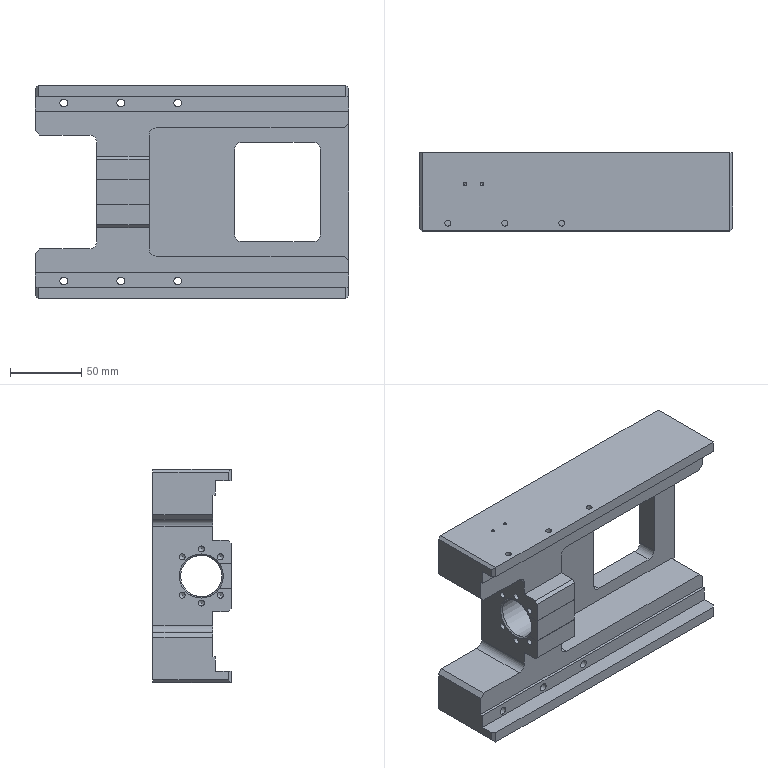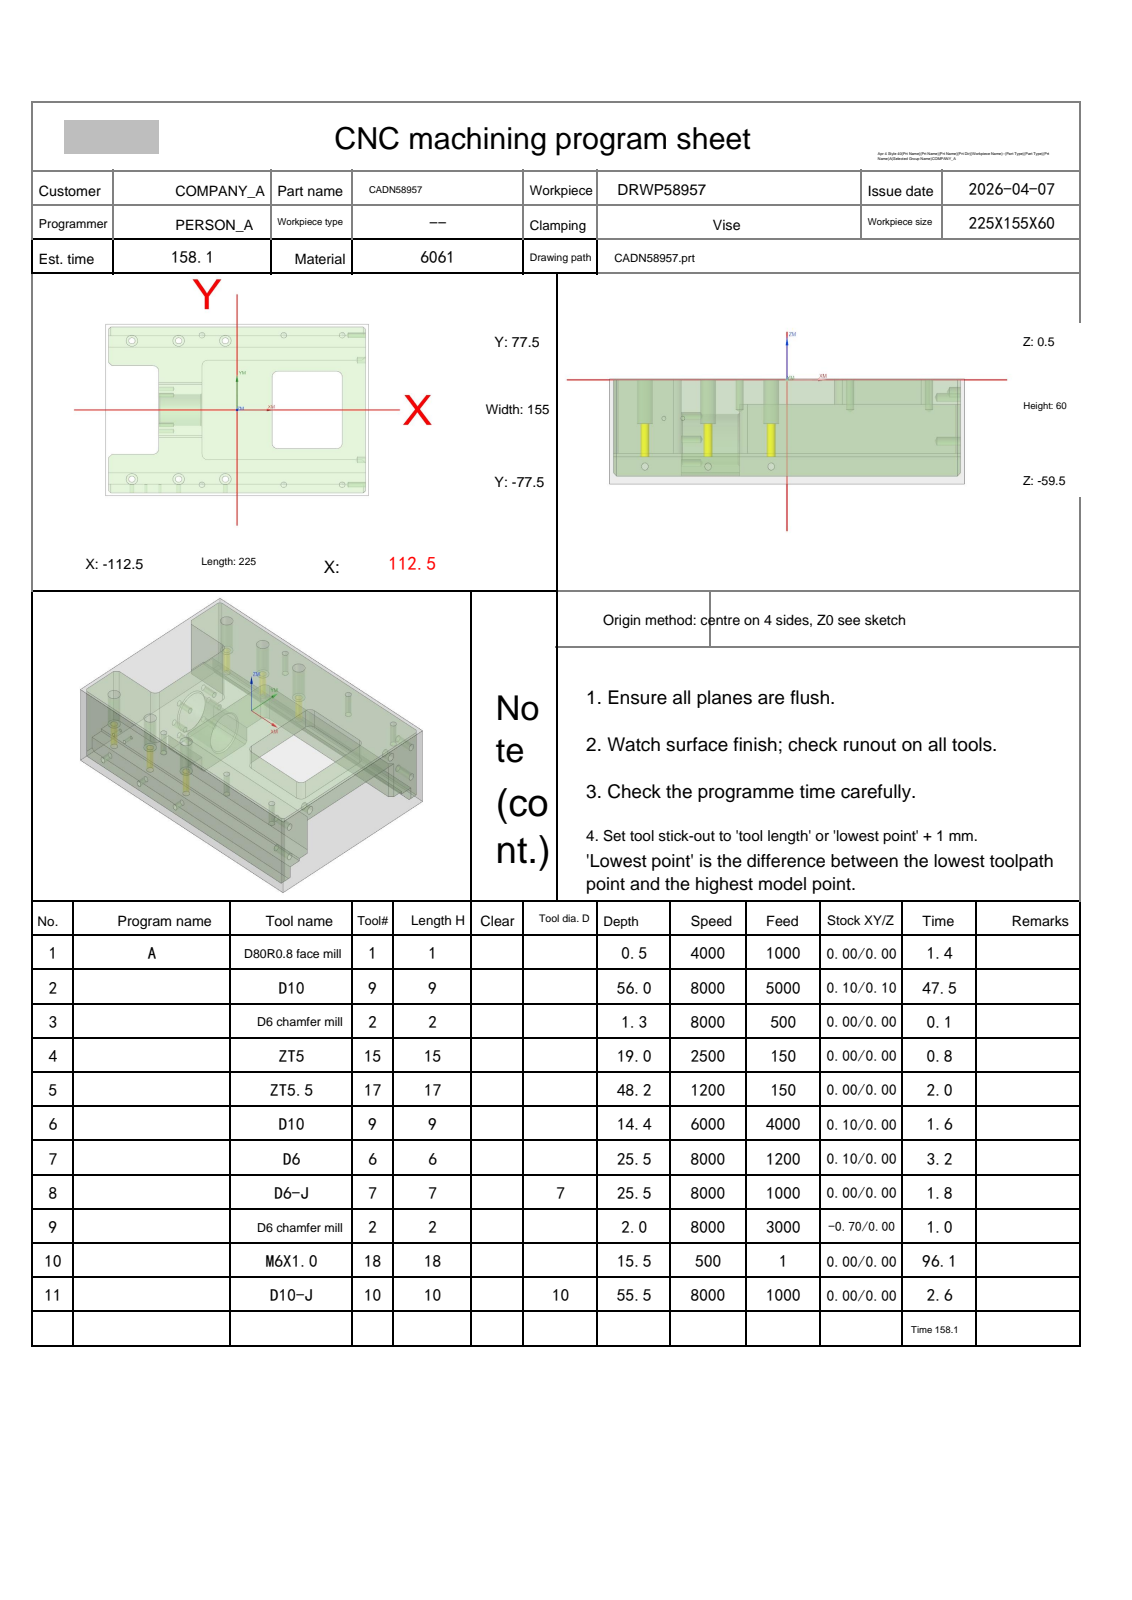NC program | NX | posted by the shop | part box 220 x 55 x 150 mm
Lines 42 to 1146 of 12878:
N2 T09 M06
(D10  D=10. R=0. H=09 ce=0.10 di=0.10)
G00 G90 G54 X-124.5 Y-7. M03 S8000
G43 H09 Z10.5
M08
Z.7
G01 Z-.5 F5000.
X-120.
G03 X-113. Y0.0 I0.0 J7.
G01 Y36.808
X-114.596 Y38.404
G02 X-116.5 Y43. I4.596 J4.596
G01 Y73.
G02 X-114.596 Y77.596 I6.5 J0.0
G01 X-112.596 Y79.596
G02 X-108. Y81.5 I4.596 J-4.596
G01 X108.
G02 X112.596 Y79.596 I0.0 J-6.5
G01 X114.596 Y77.596
G02 X116.5 Y73. I-4.596 J-4.596
G01 Y-73.
G02 X114.596 Y-77.596 I-6.5 J0.0
G01 X112.596 Y-79.596
G02 X108. Y-81.5 I-4.596 J4.596
G01 X-108.
G02 X-112.596 Y-79.596 I0.0 J6.5
G01 X-114.596 Y-77.596
G02 X-116.5 Y-73. I4.596 J4.596
G01 Y-72.99
Y-43.
G02 X-114.596 Y-38.404 I6.5 J0.0
G01 X-113. Y-36.808
Y1.986
G02 X-112.582 Y2.799 I1. J0.0
G01 X-106.418 Y7.201
G03 X-106. Y8.014 I-.582 J.813
G01 Y32.504
G02 X-105.004 Y33.5 I1. J-.004
G01 X-74.496
G02 X-73.5 Y32.504 I-.004 J-1.
G01 Y-32.504
G02 X-74.496 Y-33.5 I-1. J.004
G01 X-104.511
G03 X-105.215 Y-33.945 I0.0 J-.779
G01 X-105.383 Y-34.3
X-105.424 Y-34.48
G03 X-105.004 Y-34.9 I.42 J0.0
G01 X-72.1
Y34.9
X-107.
G02 X-110.606 Y36.394 I0.0 J5.1
G01 X-113.606 Y39.394
G02 X-115.1 Y43. I3.606 J3.606
G01 Y73.
G02 X-113.606 Y76.606 I5.1 J0.0
G01 X-111.606 Y78.606
G02 X-108. Y80.1 I3.606 J-3.606
G01 X108.
G02 X111.606 Y78.606 I0.0 J-5.1
G01 X113.606 Y76.606
G02 X115.1 Y73. I-3.606 J-3.606
G01 Y-73.
G02 X113.606 Y-76.606 I-5.1 J0.0
G01 X111.606 Y-78.606
G02 X108. Y-80.1 I-3.606 J3.606
G01 X-108.
G02 X-111.606 Y-78.606 I0.0 J5.1
G01 X-113.606 Y-76.606
G02 X-115.1 Y-73. I3.606 J3.606
G01 Y-72.99
Y-43.
G02 X-113.606 Y-39.394 I5.1 J0.0
G01 X-110.606 Y-36.394
G02 X-107. Y-34.9 I3.606 J-3.606
G01 X-105.004
G03 X-104.584 Y-34.48 I0.0 J.42
G01 X-104.624 Y-34.3
X-104.908 Y-33.702
G03 X-105.192 Y-33.481 I-.361 J-.172
G02 X-106. Y-32.504 I.192 J.981
G01 Y1.986
G02 X-105.582 Y2.799 I1. J0.0
G01 X-99.418 Y7.201
G03 X-99. Y8.014 I-.582 J.814
G01 Y25.504
G02 X-98.004 Y26.5 I1. J-.004
G01 X-81.496
G02 X-80.5 Y25.504 I-.004 J-1.
G01 Y-25.504
G02 X-81.496 Y-26.5 I-1. J.004
G01 X-98.004
G02 X-99. Y-25.504 I.004 J1.
G01 Y1.986
G02 X-98.582 Y2.799 I1. J0.0
G01 X-92.418 Y7.201
G03 X-92. Y8.014 I-.582 J.814
G01 Y18.504
G02 X-91.004 Y19.5 I1. J-.004
G01 X-88.496
G02 X-87.5 Y18.504 I-.004 J-1.
G01 Y-18.504
G02 X-88.496 Y-19.5 I-1. J.004
G01 X-91.004
G02 X-92. Y-18.504 I.004 J1.
G01 Y5.
Y5.5
G03 X-99. Y12.5 I-7. J0.0
G01 X-124.5
Z.7
G00 Z3.
G01 Y-7. F6000.
G00 Z.2
G01 Z-1. F5000.
X-120.
G03 X-113. Y0.0 I0.0 J7.
G01 Y36.808
X-114.596 Y38.404
G02 X-116.5 Y43. I4.596 J4.596
G01 Y73.
G02 X-114.596 Y77.596 I6.5 J0.0
G01 X-112.596 Y79.596
G02 X-108. Y81.5 I4.596 J-4.596
G01 X108.
G02 X112.596 Y79.596 I0.0 J-6.5
G01 X114.596 Y77.596
G02 X116.5 Y73. I-4.596 J-4.596
G01 Y-73.
G02 X114.596 Y-77.596 I-6.5 J0.0
G01 X112.596 Y-79.596
G02 X108. Y-81.5 I-4.596 J4.596
G01 X-108.
G02 X-112.596 Y-79.596 I0.0 J6.5
G01 X-114.596 Y-77.596
G02 X-116.5 Y-73. I4.596 J4.596
G01 Y-43.
G02 X-114.596 Y-38.404 I6.5 J0.0
G01 X-113. Y-36.808
Y5.
G02 X-112.238 Y5.971 I1. J0.0
G01 X-106.762 Y7.313
G03 X-106. Y8.284 I-.238 J.971
G01 Y32.503
G02 X-105.003 Y33.5 I1. J-.003
G01 X-74.497
G02 X-73.5 Y32.503 I-.003 J-1.
G01 Y-32.503
G02 X-74.497 Y-33.5 I-1. J.003
G01 X-104.511
G03 X-105.214 Y-33.945 I0.0 J-.779
G01 X-105.382 Y-34.3
X-105.423 Y-34.48
G03 X-105.003 Y-34.9 I.42 J0.0
G01 X-72.1
Y34.9
X-107.
G02 X-110.606 Y36.394 I0.0 J5.1
G01 X-113.606 Y39.394
G02 X-115.1 Y43. I3.606 J3.606
G01 Y73.
G02 X-113.606 Y76.606 I5.1 J0.0
G01 X-111.606 Y78.606
G02 X-108. Y80.1 I3.606 J-3.606
G01 X108.
G02 X111.606 Y78.606 I0.0 J-5.1
G01 X113.606 Y76.606
G02 X115.1 Y73. I-3.606 J-3.606
G01 Y-73.
G02 X113.606 Y-76.606 I-5.1 J0.0
G01 X111.606 Y-78.606
G02 X108. Y-80.1 I-3.606 J3.606
G01 X-108.
G02 X-111.606 Y-78.606 I0.0 J5.1
G01 X-113.606 Y-76.606
G02 X-115.1 Y-73. I3.606 J3.606
G01 Y-43.
G02 X-113.606 Y-39.394 I5.1 J0.0
G01 X-110.606 Y-36.394
G02 X-107. Y-34.9 I3.606 J-3.606
G01 X-105.003
G03 X-104.583 Y-34.48 I0.0 J.42
G01 X-104.624 Y-34.3
X-104.907 Y-33.702
G03 X-105.191 Y-33.482 I-.361 J-.172
G02 X-106. Y-32.503 I.191 J.982
G01 Y1.986
G02 X-105.582 Y2.799 I1. J0.0
G01 X-99.418 Y7.201
G03 X-99. Y8.014 I-.582 J.813
G01 Y25.503
G02 X-98.003 Y26.5 I1. J-.003
G01 X-81.497
G02 X-80.5 Y25.503 I-.003 J-1.
G01 Y-25.503
G02 X-81.497 Y-26.5 I-1. J.003
G01 X-98.003
G02 X-99. Y-25.503 I.003 J1.
G01 Y1.986
G02 X-98.582 Y2.799 I1. J0.0
G01 X-92.418 Y7.201
G03 X-92. Y8.014 I-.582 J.814
G01 Y18.504
G02 X-91.004 Y19.5 I1. J-.004
G01 X-88.496
G02 X-87.5 Y18.504 I-.004 J-1.
G01 Y-18.504
G02 X-88.496 Y-19.5 I-1. J.004
G01 X-91.004
G02 X-92. Y-18.504 I.004 J1.
G01 Y5.
Y5.5
G03 X-99. Y12.5 I-7. J0.0
G01 X-124.5
Z.2
G00 Z2.5
G01 Y-7. F6000.
G00 Z-.3
G01 Z-1.5 F5000.
X-120.
G03 X-113. Y0.0 I0.0 J7.
G01 Y36.808
X-114.596 Y38.404
G02 X-116.5 Y43. I4.596 J4.596
G01 Y73.
G02 X-114.596 Y77.596 I6.5 J0.0
G01 X-112.596 Y79.596
G02 X-108. Y81.5 I4.596 J-4.596
G01 X108.
G02 X112.596 Y79.596 I0.0 J-6.5
G01 X114.596 Y77.596
G02 X116.5 Y73. I-4.596 J-4.596
G01 Y-73.
G02 X114.596 Y-77.596 I-6.5 J0.0
G01 X112.596 Y-79.596
G02 X108. Y-81.5 I-4.596 J4.596
G01 X-108.
G02 X-112.596 Y-79.596 I0.0 J6.5
G01 X-114.596 Y-77.596
G02 X-116.5 Y-73. I4.596 J4.596
G01 Y-43.
G02 X-114.596 Y-38.404 I6.5 J0.0
G01 X-113. Y-36.808
Y5.
G02 X-112.238 Y5.971 I1. J0.0
G01 X-106.762 Y7.313
G03 X-106. Y8.284 I-.238 J.971
G01 Y32.503
G02 X-105.003 Y33.5 I1. J-.003
G01 X-74.497
G02 X-73.5 Y32.503 I-.003 J-1.
G01 Y-32.503
G02 X-74.497 Y-33.5 I-1. J.003
G01 X-104.511
G03 X-105.214 Y-33.945 I0.0 J-.779
G01 X-105.382 Y-34.3
X-105.423 Y-34.48
G03 X-105.003 Y-34.9 I.42 J0.0
G01 X-72.1
Y34.9
X-107.
G02 X-110.606 Y36.394 I0.0 J5.1
G01 X-113.606 Y39.394
G02 X-115.1 Y43. I3.606 J3.606
G01 Y73.
G02 X-113.606 Y76.606 I5.1 J0.0
G01 X-111.606 Y78.606
G02 X-108. Y80.1 I3.606 J-3.606
G01 X108.
G02 X111.606 Y78.606 I0.0 J-5.1
G01 X113.606 Y76.606
G02 X115.1 Y73. I-3.606 J-3.606
G01 Y-73.
G02 X113.606 Y-76.606 I-5.1 J0.0
G01 X111.606 Y-78.606
G02 X108. Y-80.1 I-3.606 J3.606
G01 X-108.
G02 X-111.606 Y-78.606 I0.0 J5.1
G01 X-113.606 Y-76.606
G02 X-115.1 Y-73. I3.606 J3.606
G01 Y-43.
G02 X-113.606 Y-39.394 I5.1 J0.0
G01 X-110.606 Y-36.394
G02 X-107. Y-34.9 I3.606 J-3.606
G01 X-105.003
G03 X-104.583 Y-34.48 I0.0 J.42
G01 X-104.624 Y-34.3
X-104.907 Y-33.702
G03 X-105.191 Y-33.482 I-.361 J-.172
G02 X-106. Y-32.503 I.191 J.982
G01 Y1.986
G02 X-105.582 Y2.799 I1. J0.0
G01 X-99.418 Y7.201
G03 X-99. Y8.014 I-.582 J.813
G01 Y25.503
G02 X-98.003 Y26.5 I1. J-.003
G01 X-81.497
G02 X-80.5 Y25.503 I-.003 J-1.
G01 Y-25.503
G02 X-81.497 Y-26.5 I-1. J.003
G01 X-98.003
G02 X-99. Y-25.503 I.003 J1.
G01 Y1.986
G02 X-98.582 Y2.799 I1. J0.0
G01 X-92.418 Y7.201
G03 X-92. Y8.014 I-.582 J.814
G01 Y18.504
G02 X-91.004 Y19.5 I1. J-.004
G01 X-88.496
G02 X-87.5 Y18.504 I-.004 J-1.
G01 Y-18.504
G02 X-88.496 Y-19.5 I-1. J.004
G01 X-91.004
G02 X-92. Y-18.504 I.004 J1.
G01 Y5.
Y5.5
G03 X-99. Y12.5 I-7. J0.0
G01 X-124.5
Z-.3
G00 Z2.
G01 Y-7. F6000.
G00 Z-.8
G01 Z-2. F5000.
X-120.
G03 X-113. Y0.0 I0.0 J7.
G01 Y36.808
X-114.596 Y38.404
G02 X-116.5 Y43. I4.596 J4.596
G01 Y73.
G02 X-114.596 Y77.596 I6.5 J0.0
G01 X-112.596 Y79.596
G02 X-108. Y81.5 I4.596 J-4.596
G01 X108.
G02 X112.596 Y79.596 I0.0 J-6.5
G01 X114.596 Y77.596
G02 X116.5 Y73. I-4.596 J-4.596
G01 Y-73.
G02 X114.596 Y-77.596 I-6.5 J0.0
G01 X112.596 Y-79.596
G02 X108. Y-81.5 I-4.596 J4.596
G01 X-108.
G02 X-112.596 Y-79.596 I0.0 J6.5
G01 X-114.596 Y-77.596
G02 X-116.5 Y-73. I4.596 J4.596
G01 Y-43.
G02 X-114.596 Y-38.404 I6.5 J0.0
G01 X-113. Y-36.808
Y5.
G02 X-112.238 Y5.971 I1. J0.0
G01 X-106.762 Y7.313
G03 X-106. Y8.284 I-.238 J.971
G01 Y32.503
G02 X-105.003 Y33.5 I1. J-.003
G01 X-74.497
G02 X-73.5 Y32.503 I-.003 J-1.
G01 Y-32.503
G02 X-74.497 Y-33.5 I-1. J.003
G01 X-104.511
G03 X-105.214 Y-33.945 I0.0 J-.779
G01 X-105.382 Y-34.3
X-105.423 Y-34.48
G03 X-105.003 Y-34.9 I.42 J0.0
G01 X-72.1
Y34.9
X-107.
G02 X-110.606 Y36.394 I0.0 J5.1
G01 X-113.606 Y39.394
G02 X-115.1 Y43. I3.606 J3.606
G01 Y73.
G02 X-113.606 Y76.606 I5.1 J0.0
G01 X-111.606 Y78.606
G02 X-108. Y80.1 I3.606 J-3.606
G01 X108.
G02 X111.606 Y78.606 I0.0 J-5.1
G01 X113.606 Y76.606
G02 X115.1 Y73. I-3.606 J-3.606
G01 Y-73.
G02 X113.606 Y-76.606 I-5.1 J0.0
G01 X111.606 Y-78.606
G02 X108. Y-80.1 I-3.606 J3.606
G01 X-108.
G02 X-111.606 Y-78.606 I0.0 J5.1
G01 X-113.606 Y-76.606
G02 X-115.1 Y-73. I3.606 J3.606
G01 Y-43.
G02 X-113.606 Y-39.394 I5.1 J0.0
G01 X-110.606 Y-36.394
G02 X-107. Y-34.9 I3.606 J-3.606
G01 X-105.003
G03 X-104.583 Y-34.48 I0.0 J.42
G01 X-104.624 Y-34.3
X-104.907 Y-33.702
G03 X-105.191 Y-33.482 I-.361 J-.172
G02 X-106. Y-32.503 I.191 J.982
G01 Y1.986
G02 X-105.582 Y2.799 I1. J0.0
G01 X-99.418 Y7.201
G03 X-99. Y8.014 I-.582 J.813
G01 Y25.503
G02 X-98.003 Y26.5 I1. J-.003
G01 X-81.497
G02 X-80.5 Y25.503 I-.003 J-1.
G01 Y-25.503
G02 X-81.497 Y-26.5 I-1. J.003
G01 X-98.003
G02 X-99. Y-25.503 I.003 J1.
G01 Y1.986
G02 X-98.582 Y2.799 I1. J0.0
G01 X-92.418 Y7.201
G03 X-92. Y8.014 I-.582 J.814
G01 Y18.504
G02 X-91.004 Y19.5 I1. J-.004
G01 X-88.496
G02 X-87.5 Y18.504 I-.004 J-1.
G01 Y-18.504
G02 X-88.496 Y-19.5 I-1. J.004
G01 X-91.004
G02 X-92. Y-18.504 I.004 J1.
G01 Y5.
Y5.5
G03 X-99. Y12.5 I-7. J0.0
G01 X-124.5
Z-.8
G00 Z1.5
G01 Y-7. F6000.
G00 Z-1.3
G01 Z-2.5 F5000.
X-120.
G03 X-113. Y0.0 I0.0 J7.
G01 Y36.808
X-114.596 Y38.404
G02 X-116.5 Y43. I4.596 J4.596
G01 Y73.
G02 X-114.596 Y77.596 I6.5 J0.0
G01 X-112.596 Y79.596
G02 X-108. Y81.5 I4.596 J-4.596
G01 X108.
G02 X112.596 Y79.596 I0.0 J-6.5
G01 X114.596 Y77.596
G02 X116.5 Y73. I-4.596 J-4.596
G01 Y-73.
G02 X114.596 Y-77.596 I-6.5 J0.0
G01 X112.596 Y-79.596
G02 X108. Y-81.5 I-4.596 J4.596
G01 X-108.
G02 X-112.596 Y-79.596 I0.0 J6.5
G01 X-114.596 Y-77.596
G02 X-116.5 Y-73. I4.596 J4.596
G01 Y-43.
G02 X-114.596 Y-38.404 I6.5 J0.0
G01 X-113. Y-36.808
Y5.
G02 X-112.238 Y5.971 I1. J0.0
G01 X-106.762 Y7.313
G03 X-106. Y8.284 I-.238 J.971
G01 Y32.503
G02 X-105.003 Y33.5 I1. J-.003
G01 X-74.497
G02 X-73.5 Y32.503 I-.003 J-1.
G01 Y-32.503
G02 X-74.497 Y-33.5 I-1. J.003
G01 X-104.511
G03 X-105.214 Y-33.945 I0.0 J-.779
G01 X-105.382 Y-34.3
X-105.423 Y-34.48
G03 X-105.003 Y-34.9 I.42 J0.0
G01 X-72.1
Y34.9
X-107.
G02 X-110.606 Y36.394 I0.0 J5.1
G01 X-113.606 Y39.394
G02 X-115.1 Y43. I3.606 J3.606
G01 Y73.
G02 X-113.606 Y76.606 I5.1 J0.0
G01 X-111.606 Y78.606
G02 X-108. Y80.1 I3.606 J-3.606
G01 X108.
G02 X111.606 Y78.606 I0.0 J-5.1
G01 X113.606 Y76.606
G02 X115.1 Y73. I-3.606 J-3.606
G01 Y-73.
G02 X113.606 Y-76.606 I-5.1 J0.0
G01 X111.606 Y-78.606
G02 X108. Y-80.1 I-3.606 J3.606
G01 X-108.
G02 X-111.606 Y-78.606 I0.0 J5.1
G01 X-113.606 Y-76.606
G02 X-115.1 Y-73. I3.606 J3.606
G01 Y-43.
G02 X-113.606 Y-39.394 I5.1 J0.0
G01 X-110.606 Y-36.394
G02 X-107. Y-34.9 I3.606 J-3.606
G01 X-105.003
G03 X-104.583 Y-34.48 I0.0 J.42
G01 X-104.624 Y-34.3
X-104.907 Y-33.702
G03 X-105.191 Y-33.482 I-.361 J-.172
G02 X-106. Y-32.503 I.191 J.982
G01 Y1.986
G02 X-105.582 Y2.799 I1. J0.0
G01 X-99.418 Y7.201
G03 X-99. Y8.014 I-.582 J.813
G01 Y25.503
G02 X-98.003 Y26.5 I1. J-.003
G01 X-81.497
G02 X-80.5 Y25.503 I-.003 J-1.
G01 Y-25.503
G02 X-81.497 Y-26.5 I-1. J.003
G01 X-98.003
G02 X-99. Y-25.503 I.003 J1.
G01 Y1.986
G02 X-98.582 Y2.799 I1. J0.0
G01 X-92.418 Y7.201
G03 X-92. Y8.014 I-.582 J.814
G01 Y18.504
G02 X-91.004 Y19.5 I1. J-.004
G01 X-88.496
G02 X-87.5 Y18.504 I-.004 J-1.
G01 Y-18.504
G02 X-88.496 Y-19.5 I-1. J.004
G01 X-91.004
G02 X-92. Y-18.504 I.004 J1.
G01 Y5.
Y5.5
G03 X-99. Y12.5 I-7. J0.0
G01 X-124.5
Z-1.3
G00 Z1.
G01 Y-7. F6000.
G00 Z-1.8
G01 Z-3. F5000.
X-120.
G03 X-113. Y0.0 I0.0 J7.
G01 Y36.808
X-114.596 Y38.404
G02 X-116.5 Y43. I4.596 J4.596
G01 Y73.
G02 X-114.596 Y77.596 I6.5 J0.0
G01 X-112.596 Y79.596
G02 X-108. Y81.5 I4.596 J-4.596
G01 X108.
G02 X112.596 Y79.596 I0.0 J-6.5
G01 X114.596 Y77.596
G02 X116.5 Y73. I-4.596 J-4.596
G01 Y-73.
G02 X114.596 Y-77.596 I-6.5 J0.0
G01 X112.596 Y-79.596
G02 X108. Y-81.5 I-4.596 J4.596
G01 X-108.
G02 X-112.596 Y-79.596 I0.0 J6.5
G01 X-114.596 Y-77.596
G02 X-116.5 Y-73. I4.596 J4.596
G01 Y-43.
G02 X-114.596 Y-38.404 I6.5 J0.0
G01 X-113. Y-36.808
Y5.
G02 X-112.238 Y5.971 I1. J0.0
G01 X-106.762 Y7.313
G03 X-106. Y8.284 I-.238 J.971
G01 Y32.503
G02 X-105.003 Y33.5 I1. J-.003
G01 X-74.497
G02 X-73.5 Y32.503 I-.003 J-1.
G01 Y-32.503
G02 X-74.497 Y-33.5 I-1. J.003
G01 X-104.511
G03 X-105.214 Y-33.945 I0.0 J-.779
G01 X-105.382 Y-34.3
X-105.423 Y-34.48
G03 X-105.003 Y-34.9 I.42 J0.0
G01 X-72.1
Y34.9
X-107.
G02 X-110.606 Y36.394 I0.0 J5.1
G01 X-113.606 Y39.394
G02 X-115.1 Y43. I3.606 J3.606
G01 Y73.
G02 X-113.606 Y76.606 I5.1 J0.0
G01 X-111.606 Y78.606
G02 X-108. Y80.1 I3.606 J-3.606
G01 X108.
G02 X111.606 Y78.606 I0.0 J-5.1
G01 X113.606 Y76.606
G02 X115.1 Y73. I-3.606 J-3.606
G01 Y-73.
G02 X113.606 Y-76.606 I-5.1 J0.0
G01 X111.606 Y-78.606
G02 X108. Y-80.1 I-3.606 J3.606
G01 X-108.
G02 X-111.606 Y-78.606 I0.0 J5.1
G01 X-113.606 Y-76.606
G02 X-115.1 Y-73. I3.606 J3.606
G01 Y-43.
G02 X-113.606 Y-39.394 I5.1 J0.0
G01 X-110.606 Y-36.394
G02 X-107. Y-34.9 I3.606 J-3.606
G01 X-105.003
G03 X-104.583 Y-34.48 I0.0 J.42
G01 X-104.624 Y-34.3
X-104.907 Y-33.702
G03 X-105.191 Y-33.482 I-.361 J-.172
G02 X-106. Y-32.503 I.191 J.982
G01 Y1.986
G02 X-105.582 Y2.799 I1. J0.0
G01 X-99.418 Y7.201
G03 X-99. Y8.014 I-.582 J.813
G01 Y25.503
G02 X-98.003 Y26.5 I1. J-.003
G01 X-81.497
G02 X-80.5 Y25.503 I-.003 J-1.
G01 Y-25.503
G02 X-81.497 Y-26.5 I-1. J.003
G01 X-98.003
G02 X-99. Y-25.503 I.003 J1.
G01 Y1.986
G02 X-98.582 Y2.799 I1. J0.0
G01 X-92.418 Y7.201
G03 X-92. Y8.014 I-.582 J.814
G01 Y18.504
G02 X-91.004 Y19.5 I1. J-.004
G01 X-88.496
G02 X-87.5 Y18.504 I-.004 J-1.
G01 Y-18.504
G02 X-88.496 Y-19.5 I-1. J.004
G01 X-91.004
G02 X-92. Y-18.504 I.004 J1.
G01 Y5.
Y5.5
G03 X-99. Y12.5 I-7. J0.0
G01 X-124.5
Z-1.8
G00 Z.5
G01 Y-7. F6000.
G00 Z-2.3
G01 Z-3.5 F5000.
X-120.
G03 X-113. Y0.0 I0.0 J7.
G01 Y36.808
X-114.596 Y38.404
G02 X-116.5 Y43. I4.596 J4.596
G01 Y73.
G02 X-114.596 Y77.596 I6.5 J0.0
G01 X-112.596 Y79.596
G02 X-108. Y81.5 I4.596 J-4.596
G01 X108.
G02 X112.596 Y79.596 I0.0 J-6.5
G01 X114.596 Y77.596
G02 X116.5 Y73. I-4.596 J-4.596
G01 Y-73.
G02 X114.596 Y-77.596 I-6.5 J0.0
G01 X112.596 Y-79.596
G02 X108. Y-81.5 I-4.596 J4.596
G01 X-108.
G02 X-112.596 Y-79.596 I0.0 J6.5
G01 X-114.596 Y-77.596
G02 X-116.5 Y-73. I4.596 J4.596
G01 Y-43.
G02 X-114.596 Y-38.404 I6.5 J0.0
G01 X-113. Y-36.808
Y5.
G02 X-112.238 Y5.971 I1. J0.0
G01 X-106.762 Y7.313
G03 X-106. Y8.284 I-.238 J.971
G01 Y32.503
G02 X-105.003 Y33.5 I1. J-.003
G01 X-74.497
G02 X-73.5 Y32.503 I-.003 J-1.
G01 Y-32.503
G02 X-74.497 Y-33.5 I-1. J.003
G01 X-104.511
G03 X-105.214 Y-33.945 I0.0 J-.779
G01 X-105.382 Y-34.3
X-105.423 Y-34.48
G03 X-105.003 Y-34.9 I.42 J0.0
G01 X-72.1
Y34.9
X-107.
G02 X-110.606 Y36.394 I0.0 J5.1
G01 X-113.606 Y39.394
G02 X-115.1 Y43. I3.606 J3.606
G01 Y73.
G02 X-113.606 Y76.606 I5.1 J0.0
G01 X-111.606 Y78.606
G02 X-108. Y80.1 I3.606 J-3.606
G01 X108.
G02 X111.606 Y78.606 I0.0 J-5.1
G01 X113.606 Y76.606
G02 X115.1 Y73. I-3.606 J-3.606
G01 Y-73.
G02 X113.606 Y-76.606 I-5.1 J0.0
G01 X111.606 Y-78.606
G02 X108. Y-80.1 I-3.606 J3.606
G01 X-108.
G02 X-111.606 Y-78.606 I0.0 J5.1
G01 X-113.606 Y-76.606
G02 X-115.1 Y-73. I3.606 J3.606
G01 Y-43.
G02 X-113.606 Y-39.394 I5.1 J0.0
G01 X-110.606 Y-36.394
G02 X-107. Y-34.9 I3.606 J-3.606
G01 X-105.003
G03 X-104.583 Y-34.48 I0.0 J.42
G01 X-104.624 Y-34.3
X-104.907 Y-33.702
G03 X-105.191 Y-33.482 I-.361 J-.172
G02 X-106. Y-32.503 I.191 J.982
G01 Y1.986
G02 X-105.582 Y2.799 I1. J0.0
G01 X-99.418 Y7.201
G03 X-99. Y8.014 I-.582 J.813
G01 Y25.503
G02 X-98.003 Y26.5 I1. J-.003
G01 X-81.497
G02 X-80.5 Y25.503 I-.003 J-1.
G01 Y-25.503
G02 X-81.497 Y-26.5 I-1. J.003
G01 X-98.003
G02 X-99. Y-25.503 I.003 J1.
G01 Y1.986
G02 X-98.582 Y2.799 I1. J0.0
G01 X-92.418 Y7.201
G03 X-92. Y8.014 I-.582 J.814
G01 Y18.504
G02 X-91.004 Y19.5 I1. J-.004
G01 X-88.496
G02 X-87.5 Y18.504 I-.004 J-1.
G01 Y-18.504
G02 X-88.496 Y-19.5 I-1. J.004
G01 X-91.004
G02 X-92. Y-18.504 I.004 J1.
G01 Y5.
Y5.5
G03 X-99. Y12.5 I-7. J0.0
G01 X-124.5
Z-2.3
G00 Z0.0
G01 Y-7. F6000.
G00 Z-2.8
G01 Z-4. F5000.
X-120.
G03 X-113. Y0.0 I0.0 J7.
G01 Y36.808
X-114.596 Y38.404
G02 X-116.5 Y43. I4.596 J4.596
G01 Y73.
G02 X-114.596 Y77.596 I6.5 J0.0
G01 X-112.596 Y79.596
G02 X-108. Y81.5 I4.596 J-4.596
G01 X108.
G02 X112.596 Y79.596 I0.0 J-6.5
G01 X114.596 Y77.596
G02 X116.5 Y73. I-4.596 J-4.596
G01 Y-73.
G02 X114.596 Y-77.596 I-6.5 J0.0
G01 X112.596 Y-79.596
G02 X108. Y-81.5 I-4.596 J4.596
G01 X-108.
G02 X-112.596 Y-79.596 I0.0 J6.5
G01 X-114.596 Y-77.596
G02 X-116.5 Y-73. I4.596 J4.596
G01 Y-43.
G02 X-114.596 Y-38.404 I6.5 J0.0
G01 X-113. Y-36.808
Y5.
G02 X-112.238 Y5.971 I1. J0.0
G01 X-106.762 Y7.313
G03 X-106. Y8.284 I-.238 J.971
G01 Y32.503
G02 X-105.003 Y33.5 I1. J-.003
G01 X-74.497
G02 X-73.5 Y32.503 I-.003 J-1.
G01 Y-32.503
G02 X-74.497 Y-33.5 I-1. J.003
G01 X-104.511
G03 X-105.214 Y-33.945 I0.0 J-.779
G01 X-105.382 Y-34.3
X-105.423 Y-34.48
G03 X-105.003 Y-34.9 I.42 J0.0
G01 X-72.1
Y34.9
X-107.
G02 X-110.606 Y36.394 I0.0 J5.1
G01 X-113.606 Y39.394
G02 X-115.1 Y43. I3.606 J3.606
G01 Y73.
G02 X-113.606 Y76.606 I5.1 J0.0
G01 X-111.606 Y78.606
G02 X-108. Y80.1 I3.606 J-3.606
G01 X108.
G02 X111.606 Y78.606 I0.0 J-5.1
G01 X113.606 Y76.606
G02 X115.1 Y73. I-3.606 J-3.606
G01 Y-73.
G02 X113.606 Y-76.606 I-5.1 J0.0
G01 X111.606 Y-78.606
G02 X108. Y-80.1 I-3.606 J3.606
G01 X-108.
G02 X-111.606 Y-78.606 I0.0 J5.1
G01 X-113.606 Y-76.606
G02 X-115.1 Y-73. I3.606 J3.606
G01 Y-43.
G02 X-113.606 Y-39.394 I5.1 J0.0
G01 X-110.606 Y-36.394
G02 X-107. Y-34.9 I3.606 J-3.606
G01 X-105.003
G03 X-104.583 Y-34.48 I0.0 J.42
G01 X-104.624 Y-34.3
X-104.907 Y-33.702
G03 X-105.191 Y-33.482 I-.361 J-.172
G02 X-106. Y-32.503 I.191 J.982
G01 Y1.986
G02 X-105.582 Y2.799 I1. J0.0
G01 X-99.418 Y7.201
G03 X-99. Y8.014 I-.582 J.813
G01 Y25.503
G02 X-98.003 Y26.5 I1. J-.003
G01 X-81.497
G02 X-80.5 Y25.503 I-.003 J-1.
G01 Y-25.503
G02 X-81.497 Y-26.5 I-1. J.003
G01 X-98.003
G02 X-99. Y-25.503 I.003 J1.
G01 Y1.986
G02 X-98.582 Y2.799 I1. J0.0
G01 X-92.418 Y7.201
G03 X-92. Y8.014 I-.582 J.814
G01 Y18.504
G02 X-91.004 Y19.5 I1. J-.004
G01 X-88.496
G02 X-87.5 Y18.504 I-.004 J-1.
G01 Y-18.504
G02 X-88.496 Y-19.5 I-1. J.004
G01 X-91.004
G02 X-92. Y-18.504 I.004 J1.
G01 Y5.
Y5.5
G03 X-99. Y12.5 I-7. J0.0
G01 X-124.5
Z-2.8
G00 Z-.5
G01 Y-7. F6000.
G00 Z-3.3
G01 Z-4.5 F5000.
X-120.
G03 X-113. Y0.0 I0.0 J7.
G01 Y36.808
X-114.596 Y38.404
G02 X-116.5 Y43. I4.596 J4.596
G01 Y73.
G02 X-114.596 Y77.596 I6.5 J0.0
G01 X-112.596 Y79.596
G02 X-108. Y81.5 I4.596 J-4.596
G01 X108.
G02 X112.596 Y79.596 I0.0 J-6.5
G01 X114.596 Y77.596
G02 X116.5 Y73. I-4.596 J-4.596
G01 Y-73.
G02 X114.596 Y-77.596 I-6.5 J0.0
G01 X112.596 Y-79.596
G02 X108. Y-81.5 I-4.596 J4.596
G01 X-108.
G02 X-112.596 Y-79.596 I0.0 J6.5
G01 X-114.596 Y-77.596
G02 X-116.5 Y-73. I4.596 J4.596
G01 Y-43.
G02 X-114.596 Y-38.404 I6.5 J0.0
G01 X-113. Y-36.808
Y5.
G02 X-112.238 Y5.971 I1. J0.0
G01 X-106.762 Y7.313
G03 X-106. Y8.284 I-.238 J.971
G01 Y32.503
G02 X-105.003 Y33.5 I1. J-.003
G01 X-74.497
G02 X-73.5 Y32.503 I-.003 J-1.
G01 Y-32.503
G02 X-74.497 Y-33.5 I-1. J.003
G01 X-104.511
G03 X-105.214 Y-33.945 I0.0 J-.779
G01 X-105.382 Y-34.3
X-105.423 Y-34.48
G03 X-105.003 Y-34.9 I.42 J0.0
G01 X-72.1
Y34.9
X-107.
G02 X-110.606 Y36.394 I0.0 J5.1
G01 X-113.606 Y39.394
G02 X-115.1 Y43. I3.606 J3.606
G01 Y73.
G02 X-113.606 Y76.606 I5.1 J0.0
G01 X-111.606 Y78.606
G02 X-108. Y80.1 I3.606 J-3.606
G01 X108.
G02 X111.606 Y78.606 I0.0 J-5.1
G01 X113.606 Y76.606
G02 X115.1 Y73. I-3.606 J-3.606
G01 Y-73.
G02 X113.606 Y-76.606 I-5.1 J0.0
G01 X111.606 Y-78.606
G02 X108. Y-80.1 I-3.606 J3.606
G01 X-108.
G02 X-111.606 Y-78.606 I0.0 J5.1
G01 X-113.606 Y-76.606
G02 X-115.1 Y-73. I3.606 J3.606
G01 Y-43.
G02 X-113.606 Y-39.394 I5.1 J0.0
G01 X-110.606 Y-36.394
G02 X-107. Y-34.9 I3.606 J-3.606
G01 X-105.003
G03 X-104.583 Y-34.48 I0.0 J.42
G01 X-104.624 Y-34.3
X-104.907 Y-33.702
G03 X-105.191 Y-33.482 I-.361 J-.172
G02 X-106. Y-32.503 I.191 J.982
G01 Y1.986
G02 X-105.582 Y2.799 I1. J0.0
G01 X-99.418 Y7.201
G03 X-99. Y8.014 I-.582 J.813
G01 Y25.503
G02 X-98.003 Y26.5 I1. J-.003
G01 X-81.497
G02 X-80.5 Y25.503 I-.003 J-1.
G01 Y-25.503
G02 X-81.497 Y-26.5 I-1. J.003
G01 X-98.003
G02 X-99. Y-25.503 I.003 J1.
G01 Y1.986
G02 X-98.582 Y2.799 I1. J0.0
G01 X-92.418 Y7.201
G03 X-92. Y8.014 I-.582 J.814
G01 Y18.504
G02 X-91.004 Y19.5 I1. J-.004
G01 X-88.496
G02 X-87.5 Y18.504 I-.004 J-1.
G01 Y-18.504
G02 X-88.496 Y-19.5 I-1. J.004
G01 X-91.004
G02 X-92. Y-18.504 I.004 J1.
G01 Y5.
Y5.5
G03 X-99. Y12.5 I-7. J0.0
G01 X-124.5
Z-3.3
G00 Z-1.
G01 Y-7. F6000.
G00 Z-3.8
G01 Z-5. F5000.
X-120.
G03 X-113. Y0.0 I0.0 J7.
G01 Y36.808
X-114.596 Y38.404
G02 X-116.5 Y43. I4.596 J4.596
G01 Y73.
G02 X-114.596 Y77.596 I6.5 J0.0
G01 X-112.596 Y79.596
G02 X-108. Y81.5 I4.596 J-4.596
G01 X108.
G02 X112.596 Y79.596 I0.0 J-6.5
G01 X114.596 Y77.596
G02 X116.5 Y73. I-4.596 J-4.596
G01 Y-73.
G02 X114.596 Y-77.596 I-6.5 J0.0
G01 X112.596 Y-79.596
G02 X108. Y-81.5 I-4.596 J4.596
G01 X-108.
G02 X-112.596 Y-79.596 I0.0 J6.5
G01 X-114.596 Y-77.596
G02 X-116.5 Y-73. I4.596 J4.596
G01 Y-43.
G02 X-114.596 Y-38.404 I6.5 J0.0
G01 X-113. Y-36.808
Y5.
G02 X-112.238 Y5.971 I1. J0.0
G01 X-106.762 Y7.313
G03 X-106. Y8.284 I-.238 J.971
G01 Y32.503
G02 X-105.003 Y33.5 I1. J-.003
G01 X-74.497
G02 X-73.5 Y32.503 I-.003 J-1.
G01 Y-32.503
G02 X-74.497 Y-33.5 I-1. J.003
G01 X-104.511
G03 X-105.214 Y-33.945 I0.0 J-.779
G01 X-105.382 Y-34.3
X-105.423 Y-34.48
G03 X-105.003 Y-34.9 I.42 J0.0
G01 X-72.1
Y34.9
X-107.
G02 X-110.606 Y36.394 I0.0 J5.1
G01 X-113.606 Y39.394
G02 X-115.1 Y43. I3.606 J3.606
G01 Y73.
G02 X-113.606 Y76.606 I5.1 J0.0
G01 X-111.606 Y78.606
G02 X-108. Y80.1 I3.606 J-3.606
G01 X108.
G02 X111.606 Y78.606 I0.0 J-5.1
G01 X113.606 Y76.606
G02 X115.1 Y73. I-3.606 J-3.606
G01 Y-73.
G02 X113.606 Y-76.606 I-5.1 J0.0
G01 X111.606 Y-78.606
G02 X108. Y-80.1 I-3.606 J3.606
G01 X-108.
G02 X-111.606 Y-78.606 I0.0 J5.1
G01 X-113.606 Y-76.606
G02 X-115.1 Y-73. I3.606 J3.606
G01 Y-43.
G02 X-113.606 Y-39.394 I5.1 J0.0
G01 X-110.606 Y-36.394
G02 X-107. Y-34.9 I3.606 J-3.606
G01 X-105.003
G03 X-104.583 Y-34.48 I0.0 J.42
G01 X-104.624 Y-34.3
X-104.907 Y-33.702
G03 X-105.191 Y-33.482 I-.361 J-.172
G02 X-106. Y-32.503 I.191 J.982
G01 Y1.986
G02 X-105.582 Y2.799 I1. J0.0
G01 X-99.418 Y7.201
G03 X-99. Y8.014 I-.582 J.813
G01 Y25.503
G02 X-98.003 Y26.5 I1. J-.003
G01 X-81.497
G02 X-80.5 Y25.503 I-.003 J-1.
G01 Y-25.503
G02 X-81.497 Y-26.5 I-1. J.003
G01 X-98.003
G02 X-99. Y-25.503 I.003 J1.
G01 Y1.986
G02 X-98.582 Y2.799 I1. J0.0
G01 X-92.418 Y7.201
G03 X-92. Y8.014 I-.582 J.814
G01 Y18.504
G02 X-91.004 Y19.5 I1. J-.004
G01 X-88.496
G02 X-87.5 Y18.504 I-.004 J-1.
G01 Y-18.504
G02 X-88.496 Y-19.5 I-1. J.004
G01 X-91.004
G02 X-92. Y-18.504 I.004 J1.
G01 Y5.
Y5.5
G03 X-99. Y12.5 I-7. J0.0
G01 X-124.5
Z-3.8
G00 Z-1.5
G01 Y-7. F6000.
G00 Z-4.3
G01 Z-5.5 F5000.
X-120.
G03 X-113. Y0.0 I0.0 J7.
G01 Y36.808
X-114.596 Y38.404
G02 X-116.5 Y43. I4.596 J4.596
G01 Y73.
G02 X-114.596 Y77.596 I6.5 J0.0
G01 X-112.596 Y79.596
G02 X-108. Y81.5 I4.596 J-4.596
G01 X108.
G02 X112.596 Y79.596 I0.0 J-6.5
G01 X114.596 Y77.596
G02 X116.5 Y73. I-4.596 J-4.596
G01 Y-73.
G02 X114.596 Y-77.596 I-6.5 J0.0
G01 X112.596 Y-79.596
G02 X108. Y-81.5 I-4.596 J4.596
G01 X-108.
G02 X-112.596 Y-79.596 I0.0 J6.5
G01 X-114.596 Y-77.596
G02 X-116.5 Y-73. I4.596 J4.596
G01 Y-43.
G02 X-114.596 Y-38.404 I6.5 J0.0
G01 X-113. Y-36.808
Y5.
G02 X-112.238 Y5.971 I1. J0.0
G01 X-106.762 Y7.313
G03 X-106. Y8.284 I-.238 J.971
G01 Y32.503
G02 X-105.003 Y33.5 I1. J-.003
G01 X-74.497
G02 X-73.5 Y32.503 I-.003 J-1.
G01 Y-32.503
G02 X-74.497 Y-33.5 I-1. J.003
G01 X-104.511
G03 X-105.214 Y-33.945 I0.0 J-.779
G01 X-105.382 Y-34.3
X-105.423 Y-34.48
G03 X-105.003 Y-34.9 I.42 J0.0
G01 X-72.1
Y34.9
X-107.
G02 X-110.606 Y36.394 I0.0 J5.1
G01 X-113.606 Y39.394
G02 X-115.1 Y43. I3.606 J3.606
G01 Y73.
G02 X-113.606 Y76.606 I5.1 J0.0
G01 X-111.606 Y78.606
G02 X-108. Y80.1 I3.606 J-3.606
G01 X108.
G02 X111.606 Y78.606 I0.0 J-5.1
G01 X113.606 Y76.606
G02 X115.1 Y73. I-3.606 J-3.606
G01 Y-73.
G02 X113.606 Y-76.606 I-5.1 J0.0
G01 X111.606 Y-78.606